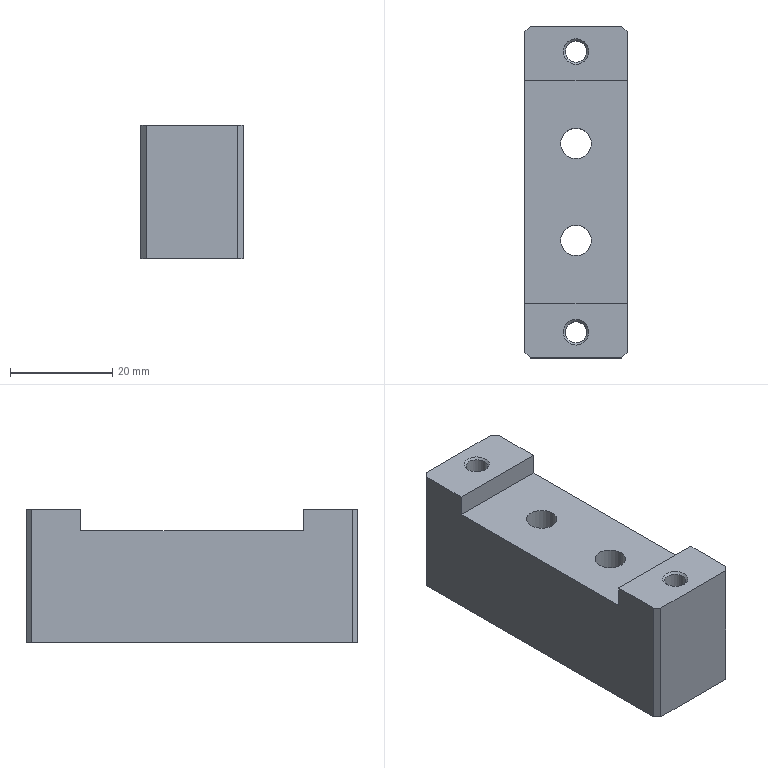Part | STEP file | Tube feed_id854_x_t | 1 solid | 22 faces | box 20 x 65 x 26.1 mm | volume 28245 mm3 | plane 14 | cylinder 4 | cone 4 | commonest cylinder face diameters 4.2 x2 6 x2